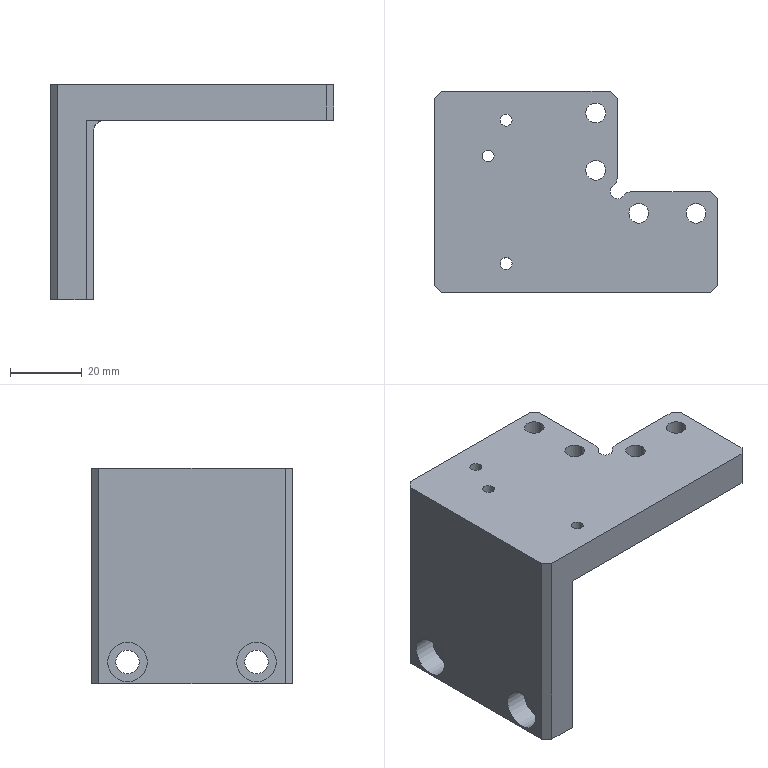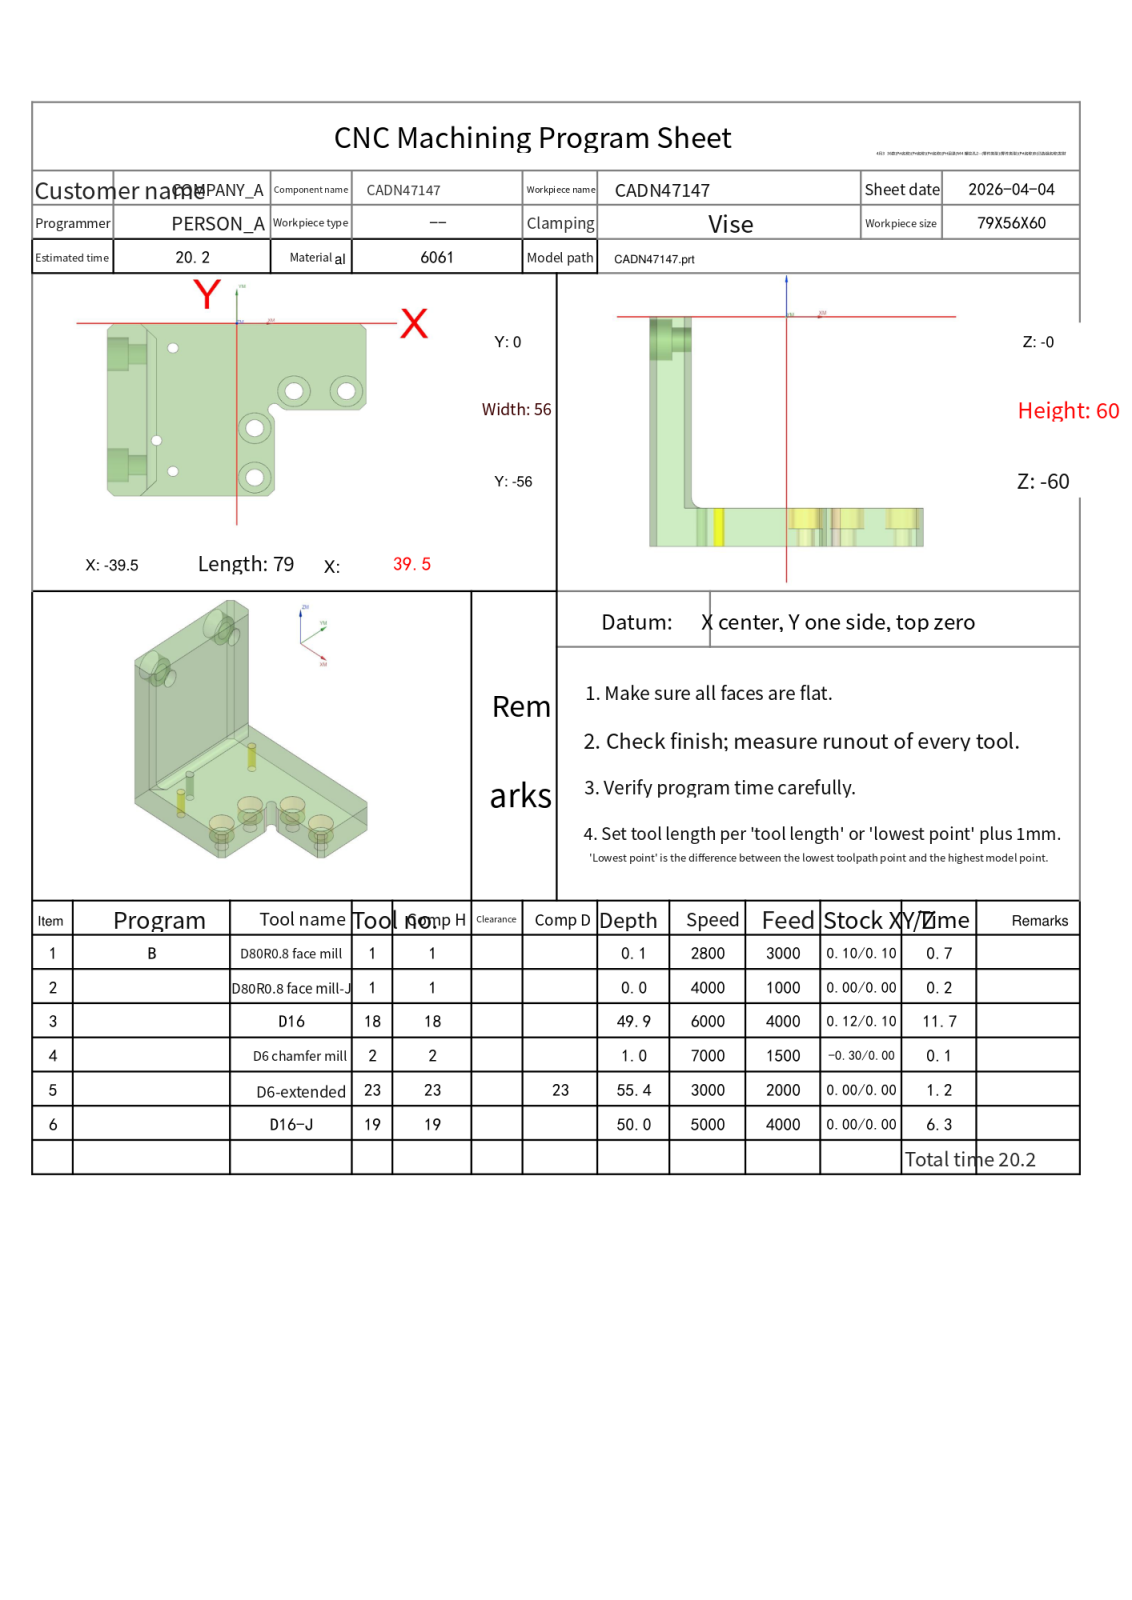NC program | NX | posted by the shop | part box 79 x 56 x 60 mm
Lines 1 to 109 of 15895:
%
O0001
(Machine time: 21.34 MIN)
(===Total Tool:5===)
(T1=D80R0.8 face mill D=80.  R=0.8  D-  H01 Z=-0.   )
(T18=D16    D=16.  R=0.   D-  H18 Z=-49.9 )
(T2=D6 chamfer mill   D=6.   R=0.   D-  H02 Z=-1.   )
(T23=D6-extended  D=6.   R=0.   D23 H23 Z=-55.4 )
(T19=D16-J  D=16.  R=0.   D19 H19 Z=-50.  )
G80 G90 G17 G49 G40
G91 G28 Z0
M01
N1 T01 M06
(D80R0.8 face mill  D=80. R=0.8 H=01 ce=0.10 di=0.10)
G00 G90 G54 X91.597 Y-28. M03 S2800
G43 H01 Z20.
M08
Z6.011
G01 Z4.011 F3000.
X79.597
X-79.597
X-91.597
Z6.011
G00 X91.597
Z5.522
G01 Z3.522
X79.597
X-79.597
X-91.597
Z5.522
G00 X91.597
Z5.033
G01 Z3.033
X79.597
X-79.597
X-91.597
Z5.033
G00 X91.597
Z4.544
G01 Z2.544
X79.597
X-79.597
X-91.597
Z4.544
G00 Z20.
X91.597
Z4.056
G01 Z2.056
X79.597
X-79.597
X-91.597
Z4.056
G00 Z20.
X91.597
Z3.567
G01 Z1.567
X79.597
X-79.597
X-91.597
Z3.567
G00 Z20.
X91.597
Z3.078
G01 Z1.078
X79.597
X-79.597
X-91.597
Z3.078
G00 Z20.
X91.597
Z2.589
G01 Z.589
X79.597
X-79.597
X-91.597
Z2.589
G00 Z20.
X91.597
Z2.1
G01 Z.1
X79.597
X-79.597
X-91.597
Z2.1
G00 Z20.
G91 G28 Z0.0
M05
M09
G91 G28 Z0.0
M01
N2 T01 M06
(D80R0.8 face mill-J  D=80. R=0.8 H=01 ce=0.00 di=0.00)
G00 G90 G54 X91.499 Y-28. M03 S4000
G43 H01 Z20.
M08
Z2.
G01 Z0.0 F1000.
X79.499
X-79.499
X-91.499
Z2.
G00 Z20.
G91 G28 Z0.0
M05
M09
G91 G28 Z0.0
M01